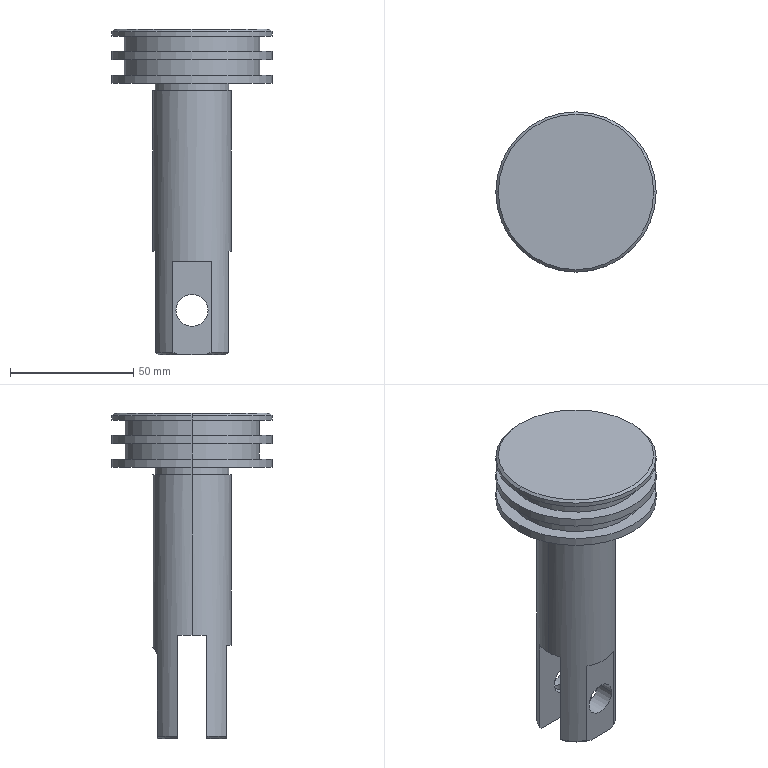Part | SolidWorks | features ICE 9, Chamfer 2, 3DProfileFeature 1, Extrusion 1, Fillet 1, HoleWzd 1 | 1 solid | 42 faces | box 65 x 65 x 132 mm | volume 129865 mm3 | cylinder 21 | plane 15 | cone 6 | commonest cylinder face diameters 65 x6 13 x4 55 x4 3.3 x2 30 x2 32 x2
STEP:
#1=CARTESIAN_POINT('',(1.65,10.,-98.287));
#2=VERTEX_POINT('',#1);
#3=CARTESIAN_POINT('',(-1.65,10.,-98.287));
#4=VERTEX_POINT('',#3);
#5=CARTESIAN_POINT('',(1.65,10.,-98.287));
#6=CARTESIAN_POINT('',(1.65,9.784,-98.287));
#7=CARTESIAN_POINT('',(1.606,9.566,-98.299));
#8=CARTESIAN_POINT('',(1.483,9.268,-98.329));
#9=CARTESIAN_POINT('',(1.431,9.172,-98.341));
#10=CARTESIAN_POINT('',(1.311,8.993,-98.367));
#11=CARTESIAN_POINT('',(1.243,8.91,-98.38));
#12=CARTESIAN_POINT('',(1.091,8.758,-98.408));
#13=CARTESIAN_POINT('',(1.007,8.688,-98.422));
#14=CARTESIAN_POINT('',(0.8287,8.569,-98.448));
#15=CARTESIAN_POINT('',(0.7341,8.518,-98.459));
#16=CARTESIAN_POINT('',(0.4329,8.393,-98.489));
#17=CARTESIAN_POINT('',(0.2181,8.35,-98.5));
#18=CARTESIAN_POINT('',(-0.1083,8.35,-98.5));
#19=CARTESIAN_POINT('',(-0.2157,8.361,-98.497));
#20=CARTESIAN_POINT('',(-0.4277,8.403,-98.487));
#21=CARTESIAN_POINT('',(-0.533,8.435,-98.479));
#22=CARTESIAN_POINT('',(-0.8316,8.559,-98.45));
#23=CARTESIAN_POINT('',(-1.015,8.681,-98.422));
#24=CARTESIAN_POINT('',(-1.318,8.984,-98.367));
#25=CARTESIAN_POINT('',(-1.44,9.167,-98.339));
#26=CARTESIAN_POINT('',(-1.565,9.465,-98.309));
#27=CARTESIAN_POINT('',(-1.597,9.57,-98.301));
#28=CARTESIAN_POINT('',(-1.639,9.783,-98.29));
#29=CARTESIAN_POINT('',(-1.65,9.891,-98.287));
#30=CARTESIAN_POINT('',(-1.65,10.,-98.287));
#31=B_SPLINE_CURVE_WITH_KNOTS('',3,(#5,#6,#7,#8,#9,#10,#11,#12,#13,#14,#15,#16,#17,#18,#19,#20,#21,#22,#23,#24,#25,#26,#27,#28,#29,#30),.UNSPECIFIED.,.F.,.F.,(4,2,2,2,2,2,2,2,2,2,2,2,4),(0.00518,0.005827,0.006151,0.006474,0.006798,0.007122,0.007769,0.008093,0.008416,0.009064,0.009711,0.01003,0.01036),.UNSPECIFIED.);
#32=EDGE_CURVE('',#2,#4,#31,.T.);
#33=ORIENTED_EDGE('',*,*,#32,.F.);
#34=CARTESIAN_POINT('',(1.65,10.,-110.));
#35=VERTEX_POINT('',#34);
#36=CARTESIAN_POINT('',(1.65,10.,-110.));
#37=DIRECTION('',(0.,0.,-1.));
#38=VECTOR('',#37,1000.);
#39=LINE('',#36,#38);
#40=EDGE_CURVE('',#2,#35,#39,.T.);
#41=ORIENTED_EDGE('',*,*,#40,.T.);
#42=CARTESIAN_POINT('',(-1.65,10.,-110.));
#43=VERTEX_POINT('',#42);
#44=CARTESIAN_POINT('',(0.,10.,-110.));
#45=DIRECTION('',(0.,0.,-1.));
#46=DIRECTION('',(-1.,0.,0.));
#47=AXIS2_PLACEMENT_3D('',#44,#45,#46);
#48=CIRCLE('',#47,1.65);
#49=EDGE_CURVE('',#35,#43,#48,.T.);
#50=ORIENTED_EDGE('',*,*,#49,.T.);
#51=CARTESIAN_POINT('',(-1.65,10.,-110.));
#52=DIRECTION('',(0.,0.,-1.));
#53=VECTOR('',#52,1000.);
#54=LINE('',#51,#53);
#55=EDGE_CURVE('',#4,#43,#54,.T.);
#56=ORIENTED_EDGE('',*,*,#55,.F.);
#57=EDGE_LOOP('',(#33,#41,#50,#56));
#58=FACE_OUTER_BOUND('',#57,.T.);
#59=CARTESIAN_POINT('',(0.,10.,-110.));
#60=DIRECTION('',(0.,0.,-1.));
#61=DIRECTION('',(-1.,0.,0.));
#62=AXIS2_PLACEMENT_3D('',#59,#60,#61);
#63=CYLINDRICAL_SURFACE('',#62,1.65);
#64=ADVANCED_FACE('',(#58),#63,.F.);
#65=CARTESIAN_POINT('',(6.5,-14.,-92.));
#66=VERTEX_POINT('',#65);
#67=CARTESIAN_POINT('',(-6.5,-14.,-92.));
#68=VERTEX_POINT('',#67);
#69=CARTESIAN_POINT('',(0.,-14.,-92.));
#70=DIRECTION('',(0.,1.,0.));
#71=DIRECTION('',(-1.,0.,0.));
#72=AXIS2_PLACEMENT_3D('',#69,#70,#71);
#73=CIRCLE('',#72,6.5);
#74=EDGE_CURVE('',#66,#68,#73,.T.);
#75=ORIENTED_EDGE('',*,*,#74,.F.);
#76=CARTESIAN_POINT('',(6.5,-6.,-92.));
#77=VERTEX_POINT('',#76);
#78=CARTESIAN_POINT('',(6.5,-32.5,-92.));
#79=DIRECTION('',(0.,1.,0.));
#80=VECTOR('',#79,1000.);
#81=LINE('',#78,#80);
#82=EDGE_CURVE('',#66,#77,#81,.T.);
#83=ORIENTED_EDGE('',*,*,#82,.T.);
#84=CARTESIAN_POINT('',(-6.5,-6.,-92.));
#85=VERTEX_POINT('',#84);
#86=CARTESIAN_POINT('',(0.,-6.,-92.));
#87=DIRECTION('',(0.,-1.,0.));
#88=DIRECTION('',(1.,0.,0.));
#89=AXIS2_PLACEMENT_3D('',#86,#87,#88);
#90=CIRCLE('',#89,6.5);
#91=EDGE_CURVE('',#85,#77,#90,.T.);
#92=ORIENTED_EDGE('',*,*,#91,.F.);
#93=CARTESIAN_POINT('',(-6.5,-32.5,-92.));
#94=DIRECTION('',(0.,1.,0.));
#95=VECTOR('',#94,1000.);
#96=LINE('',#93,#95);
#97=EDGE_CURVE('',#68,#85,#96,.T.);
#98=ORIENTED_EDGE('',*,*,#97,.F.);
#99=EDGE_LOOP('',(#75,#83,#92,#98));
#100=FACE_OUTER_BOUND('',#99,.T.);
#101=CARTESIAN_POINT('',(0.,-32.5,-92.));
#102=DIRECTION('',(0.,1.,0.));
#103=DIRECTION('',(-1.,0.,0.));
#104=AXIS2_PLACEMENT_3D('',#101,#102,#103);
#105=CYLINDRICAL_SURFACE('',#104,6.5);
#106=ADVANCED_FACE('',(#100),#105,.F.);
#107=CARTESIAN_POINT('',(-1.65,10.,-98.287));
#108=CARTESIAN_POINT('',(-1.65,10.11,-98.287));
#109=CARTESIAN_POINT('',(-1.639,10.217,-98.29));
#110=CARTESIAN_POINT('',(-1.597,10.429,-98.301));
#111=CARTESIAN_POINT('',(-1.565,10.534,-98.309));
#112=CARTESIAN_POINT('',(-1.482,10.733,-98.329));
#113=CARTESIAN_POINT('',(-1.431,10.828,-98.341));
#114=CARTESIAN_POINT('',(-1.312,11.007,-98.367));
#115=CARTESIAN_POINT('',(-1.242,11.091,-98.381));
#116=CARTESIAN_POINT('',(-1.015,11.318,-98.422));
#117=CARTESIAN_POINT('',(-0.8315,11.441,-98.45));
#118=CARTESIAN_POINT('',(-0.4347,11.606,-98.489));
#119=CARTESIAN_POINT('',(-0.2169,11.65,-98.5));
#120=CARTESIAN_POINT('',(0.1074,11.65,-98.5));
#121=CARTESIAN_POINT('',(0.2173,11.639,-98.497));
#122=CARTESIAN_POINT('',(0.4293,11.597,-98.487));
#123=CARTESIAN_POINT('',(0.5324,11.566,-98.479));
#124=CARTESIAN_POINT('',(0.8329,11.441,-98.45));
#125=CARTESIAN_POINT('',(1.014,11.319,-98.422));
#126=CARTESIAN_POINT('',(1.243,11.09,-98.38));
#127=CARTESIAN_POINT('',(1.311,11.007,-98.367));
#128=CARTESIAN_POINT('',(1.431,10.829,-98.341));
#129=CARTESIAN_POINT('',(1.483,10.732,-98.329));
#130=CARTESIAN_POINT('',(1.565,10.533,-98.309));
#131=CARTESIAN_POINT('',(1.597,10.43,-98.301));
#132=CARTESIAN_POINT('',(1.639,10.218,-98.29));
#133=CARTESIAN_POINT('',(1.65,10.108,-98.287));
#134=CARTESIAN_POINT('',(1.65,10.,-98.287));
#135=B_SPLINE_CURVE_WITH_KNOTS('',3,(#107,#108,#109,#110,#111,#112,#113,#114,#115,#116,#117,#118,#119,#120,#121,#122,#123,#124,#125,#126,#127,#128,#129,#130,#131,#132,#133,#134),.UNSPECIFIED.,.F.,.F.,(4,2,2,2,2,2,2,2,2,2,2,2,2,4),(0.,0.0003237,0.0006475,0.0009712,0.001295,0.001942,0.00259,0.002914,0.003237,0.003885,0.004209,0.004532,0.004856,0.00518),.UNSPECIFIED.);
#136=EDGE_CURVE('',#4,#2,#135,.T.);
#137=ORIENTED_EDGE('',*,*,#136,.T.);
#138=ORIENTED_EDGE('',*,*,#32,.T.);
#139=EDGE_LOOP('',(#137,#138));
#140=FACE_BOUND('',#139,.T.);
#141=CARTESIAN_POINT('',(6.5,6.,-92.));
#142=VERTEX_POINT('',#141);
#143=CARTESIAN_POINT('',(-6.5,6.,-92.));
#144=VERTEX_POINT('',#143);
#145=CARTESIAN_POINT('',(0.,6.,-92.));
#146=DIRECTION('',(0.,1.,0.));
#147=DIRECTION('',(-1.,0.,0.));
#148=AXIS2_PLACEMENT_3D('',#145,#146,#147);
#149=CIRCLE('',#148,6.5);
#150=EDGE_CURVE('',#142,#144,#149,.T.);
#151=ORIENTED_EDGE('',*,*,#150,.F.);
#152=CARTESIAN_POINT('',(6.5,14.,-92.));
#153=VERTEX_POINT('',#152);
#154=CARTESIAN_POINT('',(6.5,-32.5,-92.));
#155=DIRECTION('',(0.,1.,0.));
#156=VECTOR('',#155,1000.);
#157=LINE('',#154,#156);
#158=EDGE_CURVE('',#142,#153,#157,.T.);
#159=ORIENTED_EDGE('',*,*,#158,.T.);
#160=CARTESIAN_POINT('',(-6.5,14.,-92.));
#161=VERTEX_POINT('',#160);
#162=CARTESIAN_POINT('',(0.,14.,-92.));
#163=DIRECTION('',(0.,1.,0.));
#164=DIRECTION('',(-1.,0.,0.));
#165=AXIS2_PLACEMENT_3D('',#162,#163,#164);
#166=CIRCLE('',#165,6.5);
#167=EDGE_CURVE('',#153,#161,#166,.T.);
#168=ORIENTED_EDGE('',*,*,#167,.T.);
#169=CARTESIAN_POINT('',(-6.5,-32.5,-92.));
#170=DIRECTION('',(0.,1.,0.));
#171=VECTOR('',#170,1000.);
#172=LINE('',#169,#171);
#173=EDGE_CURVE('',#144,#161,#172,.T.);
#174=ORIENTED_EDGE('',*,*,#173,.F.);
#175=EDGE_LOOP('',(#151,#159,#168,#174));
#176=FACE_OUTER_BOUND('',#175,.T.);
#177=CARTESIAN_POINT('',(0.,-32.5,-92.));
#178=DIRECTION('',(0.,1.,0.));
#179=DIRECTION('',(-1.,0.,0.));
#180=AXIS2_PLACEMENT_3D('',#177,#178,#179);
#181=CYLINDRICAL_SURFACE('',#180,6.5);
#182=ADVANCED_FACE('',(#140,#176),#181,.F.);
#183=CARTESIAN_POINT('',(-16.,0.,-68.));
#184=VERTEX_POINT('',#183);
#185=CARTESIAN_POINT('',(-14.832,6.,-68.));
#186=VERTEX_POINT('',#185);
#187=CARTESIAN_POINT('',(0.,0.,-68.));
#188=DIRECTION('',(0.,0.,-1.));
#189=DIRECTION('',(-1.,0.,0.));
#190=AXIS2_PLACEMENT_3D('',#187,#188,#189);
#191=CIRCLE('',#190,16.);
#192=EDGE_CURVE('',#184,#186,#191,.T.);
#193=ORIENTED_EDGE('',*,*,#192,.F.);
#194=CARTESIAN_POINT('',(-16.,0.,-3.));
#195=VERTEX_POINT('',#194);
#196=CARTESIAN_POINT('',(-16.,0.,-110.));
#197=DIRECTION('',(0.,0.,1.));
#198=VECTOR('',#197,1000.);
#199=LINE('',#196,#198);
#200=EDGE_CURVE('',#184,#195,#199,.T.);
#201=ORIENTED_EDGE('',*,*,#200,.T.);
#202=CARTESIAN_POINT('',(16.,0.,-3.));
#203=VERTEX_POINT('',#202);
#204=CARTESIAN_POINT('',(0.,0.,-3.));
#205=DIRECTION('',(0.,0.,-1.));
#206=DIRECTION('',(-1.,0.,0.));
#207=AXIS2_PLACEMENT_3D('',#204,#205,#206);
#208=CIRCLE('',#207,16.);
#209=EDGE_CURVE('',#195,#203,#208,.T.);
#210=ORIENTED_EDGE('',*,*,#209,.T.);
#211=CARTESIAN_POINT('',(16.,0.,-68.));
#212=VERTEX_POINT('',#211);
#213=CARTESIAN_POINT('',(16.,0.,-110.));
#214=DIRECTION('',(0.,0.,1.));
#215=VECTOR('',#214,1000.);
#216=LINE('',#213,#215);
#217=EDGE_CURVE('',#212,#203,#216,.T.);
#218=ORIENTED_EDGE('',*,*,#217,.F.);
#219=CARTESIAN_POINT('',(14.832,6.,-68.));
#220=VERTEX_POINT('',#219);
#221=CARTESIAN_POINT('',(0.,0.,-68.));
#222=DIRECTION('',(0.,0.,-1.));
#223=DIRECTION('',(-1.,0.,0.));
#224=AXIS2_PLACEMENT_3D('',#221,#222,#223);
#225=CIRCLE('',#224,16.);
#226=EDGE_CURVE('',#220,#212,#225,.T.);
#227=ORIENTED_EDGE('',*,*,#226,.F.);
#228=CARTESIAN_POINT('',(14.832,6.,-109.));
#229=VERTEX_POINT('',#228);
#230=CARTESIAN_POINT('',(14.832,6.,-110.));
#231=DIRECTION('',(0.,0.,-1.));
#232=VECTOR('',#231,1000.);
#233=LINE('',#230,#232);
#234=EDGE_CURVE('',#220,#229,#233,.T.);
#235=ORIENTED_EDGE('',*,*,#234,.T.);
#236=CARTESIAN_POINT('',(7.746,14.,-109.));
#237=VERTEX_POINT('',#236);
#238=CARTESIAN_POINT('',(0.,0.,-109.));
#239=DIRECTION('',(0.,0.,1.));
#240=DIRECTION('',(-1.,0.,0.));
#241=AXIS2_PLACEMENT_3D('',#238,#239,#240);
#242=CIRCLE('',#241,16.);
#243=EDGE_CURVE('',#229,#237,#242,.T.);
#244=ORIENTED_EDGE('',*,*,#243,.T.);
#245=CARTESIAN_POINT('',(7.746,14.,-77.));
#246=VERTEX_POINT('',#245);
#247=CARTESIAN_POINT('',(7.746,14.,-110.));
#248=DIRECTION('',(0.,0.,1.));
#249=VECTOR('',#248,1000.);
#250=LINE('',#247,#249);
#251=EDGE_CURVE('',#237,#246,#250,.T.);
#252=ORIENTED_EDGE('',*,*,#251,.T.);
#253=CARTESIAN_POINT('',(-7.746,14.,-77.));
#254=VERTEX_POINT('',#253);
#255=CARTESIAN_POINT('',(7.746,14.,-77.));
#256=CARTESIAN_POINT('',(7.746,14.,-76.791));
#257=CARTESIAN_POINT('',(7.722,14.013,-76.586));
#258=CARTESIAN_POINT('',(7.632,14.063,-76.186));
#259=CARTESIAN_POINT('',(7.564,14.099,-75.99));
#260=CARTESIAN_POINT('',(7.394,14.189,-75.624));
#261=CARTESIAN_POINT('',(7.291,14.243,-75.451));
#262=CARTESIAN_POINT('',(7.057,14.36,-75.129));
#263=CARTESIAN_POINT('',(6.928,14.423,-74.982));
#264=CARTESIAN_POINT('',(6.65,14.554,-74.708));
#265=CARTESIAN_POINT('',(6.499,14.622,-74.582));
#266=CARTESIAN_POINT('',(6.184,14.758,-74.35));
#267=CARTESIAN_POINT('',(6.02,14.825,-74.246));
#268=CARTESIAN_POINT('',(5.514,15.024,-73.959));
#269=CARTESIAN_POINT('',(5.155,15.152,-73.803));
#270=CARTESIAN_POINT('',(4.406,15.386,-73.54));
#271=CARTESIAN_POINT('',(4.024,15.491,-73.436));
#272=CARTESIAN_POINT('',(3.245,15.672,-73.266));
#273=CARTESIAN_POINT('',(2.85,15.749,-73.2));
#274=CARTESIAN_POINT('',(2.047,15.874,-73.097));
#275=CARTESIAN_POINT('',(1.638,15.921,-73.06));
#276=CARTESIAN_POINT('',(0.8181,15.984,-73.012));
#277=CARTESIAN_POINT('',(0.4067,16.,-73.));
#278=CARTESIAN_POINT('',(-0.8311,16.,-73.));
#279=CARTESIAN_POINT('',(-1.643,15.936,-73.046));
#280=CARTESIAN_POINT('',(-2.839,15.751,-73.198));
#281=CARTESIAN_POINT('',(-3.235,15.675,-73.264));
#282=CARTESIAN_POINT('',(-4.017,15.493,-73.434));
#283=CARTESIAN_POINT('',(-4.405,15.387,-73.54));
#284=CARTESIAN_POINT('',(-5.15,15.154,-73.801));
#285=CARTESIAN_POINT('',(-5.511,15.026,-73.957));
#286=CARTESIAN_POINT('',(-6.192,14.758,-74.343));
#287=CARTESIAN_POINT('',(-6.507,14.62,-74.569));
#288=CARTESIAN_POINT('',(-6.927,14.424,-74.98));
#289=CARTESIAN_POINT('',(-7.058,14.36,-75.13));
#290=CARTESIAN_POINT('',(-7.29,14.243,-75.45));
#291=CARTESIAN_POINT('',(-7.392,14.19,-75.621));
#292=CARTESIAN_POINT('',(-7.564,14.099,-75.99));
#293=CARTESIAN_POINT('',(-7.631,14.063,-76.182));
#294=CARTESIAN_POINT('',(-7.722,14.013,-76.582));
#295=CARTESIAN_POINT('',(-7.746,14.,-76.791));
#296=CARTESIAN_POINT('',(-7.746,14.,-77.));
#297=B_SPLINE_CURVE_WITH_KNOTS('',3,(#255,#256,#257,#258,#259,#260,#261,#262,#263,#264,#265,#266,#267,#268,#269,#270,#271,#272,#273,#274,#275,#276,#277,#278,#279,#280,#281,#282,#283,#284,#285,#286,#287,#288,#289,#290,#291,#292,#293,#294,#295,#296),.UNSPECIFIED.,.F.,.F.,(4,2,2,2,2,2,2,2,2,2,2,2,2,2,2,2,2,2,2,2,4),(-0.009753,-0.009143,-0.008533,-0.007923,-0.007313,-0.006703,-0.006093,-0.004873,-0.003654,-0.002434,-0.001214,0.000005848,0.002446,0.003665,0.004885,0.006105,0.007325,0.007935,0.008545,0.009155,0.009765),.UNSPECIFIED.);
#298=EDGE_CURVE('',#246,#254,#297,.T.);
#299=ORIENTED_EDGE('',*,*,#298,.T.);
#300=CARTESIAN_POINT('',(-7.746,14.,-109.));
#301=VERTEX_POINT('',#300);
#302=CARTESIAN_POINT('',(-7.746,14.,-110.));
#303=DIRECTION('',(0.,0.,-1.));
#304=VECTOR('',#303,1000.);
#305=LINE('',#302,#304);
#306=EDGE_CURVE('',#254,#301,#305,.T.);
#307=ORIENTED_EDGE('',*,*,#306,.T.);
#308=CARTESIAN_POINT('',(-14.832,6.,-109.));
#309=VERTEX_POINT('',#308);
#310=CARTESIAN_POINT('',(0.,0.,-109.));
#311=DIRECTION('',(0.,0.,1.));
#312=DIRECTION('',(-1.,0.,0.));
#313=AXIS2_PLACEMENT_3D('',#310,#311,#312);
#314=CIRCLE('',#313,16.);
#315=EDGE_CURVE('',#301,#309,#314,.T.);
#316=ORIENTED_EDGE('',*,*,#315,.T.);
#317=CARTESIAN_POINT('',(-14.832,6.,-110.));
#318=DIRECTION('',(0.,0.,1.));
#319=VECTOR('',#318,1000.);
#320=LINE('',#317,#319);
#321=EDGE_CURVE('',#309,#186,#320,.T.);
#322=ORIENTED_EDGE('',*,*,#321,.T.);
#323=EDGE_LOOP('',(#193,#201,#210,#218,#227,#235,#244,#252,#299,#307,#316,#322));
#324=FACE_OUTER_BOUND('',#323,.T.);
#325=CARTESIAN_POINT('',(0.,0.,-110.));
#326=DIRECTION('',(0.,0.,1.));
#327=DIRECTION('',(1.,0.,0.));
#328=AXIS2_PLACEMENT_3D('',#325,#326,#327);
#329=CYLINDRICAL_SURFACE('',#328,16.);
#330=ADVANCED_FACE('',(#324),#329,.T.);
#331=CARTESIAN_POINT('',(-15.,0.,-3.));
#332=VERTEX_POINT('',#331);
#333=CARTESIAN_POINT('',(15.,0.,-3.));
#334=VERTEX_POINT('',#333);
#335=CARTESIAN_POINT('',(0.,0.,-3.));
#336=DIRECTION('',(0.,0.,-1.));
#337=DIRECTION('',(-1.,0.,0.));
#338=AXIS2_PLACEMENT_3D('',#335,#336,#337);
#339=CIRCLE('',#338,15.);
#340=EDGE_CURVE('',#332,#334,#339,.T.);
#341=ORIENTED_EDGE('',*,*,#340,.F.);
#342=CARTESIAN_POINT('',(-15.,0.,0.));
#343=VERTEX_POINT('',#342);
#344=CARTESIAN_POINT('',(-15.,0.,-3.));
#345=DIRECTION('',(0.,0.,1.));
#346=VECTOR('',#345,1000.);
#347=LINE('',#344,#346);
#348=EDGE_CURVE('',#332,#343,#347,.T.);
#349=ORIENTED_EDGE('',*,*,#348,.T.);
#350=CARTESIAN_POINT('',(15.,0.,0.));
#351=VERTEX_POINT('',#350);
#352=CARTESIAN_POINT('',(0.,0.,0.));
#353=DIRECTION('',(0.,0.,-1.));
#354=DIRECTION('',(-1.,0.,0.));
#355=AXIS2_PLACEMENT_3D('',#352,#353,#354);
#356=CIRCLE('',#355,15.);
#357=EDGE_CURVE('',#343,#351,#356,.T.);
#358=ORIENTED_EDGE('',*,*,#357,.T.);
#359=CARTESIAN_POINT('',(15.,0.,-3.));
#360=DIRECTION('',(0.,0.,1.));
#361=VECTOR('',#360,1000.);
#362=LINE('',#359,#361);
#363=EDGE_CURVE('',#334,#351,#362,.T.);
#364=ORIENTED_EDGE('',*,*,#363,.F.);
#365=EDGE_LOOP('',(#341,#349,#358,#364));
#366=FACE_OUTER_BOUND('',#365,.T.);
#367=CARTESIAN_POINT('',(0.,0.,-3.));
#368=DIRECTION('',(0.,0.,1.));
#369=DIRECTION('',(1.,0.,0.));
#370=AXIS2_PLACEMENT_3D('',#367,#368,#369);
#371=CYLINDRICAL_SURFACE('',#370,15.);
#372=ADVANCED_FACE('',(#366),#371,.T.);
#373=CARTESIAN_POINT('',(31.5,0.,22.));
#374=VERTEX_POINT('',#373);
#375=CARTESIAN_POINT('',(-31.5,0.,22.));
#376=VERTEX_POINT('',#375);
#377=CARTESIAN_POINT('',(0.,0.,22.));
#378=DIRECTION('',(0.,0.,1.));
#379=DIRECTION('',(1.,0.,0.));
#380=AXIS2_PLACEMENT_3D('',#377,#378,#379);
#381=CIRCLE('',#380,31.5);
#382=EDGE_CURVE('',#374,#376,#381,.T.);
#383=ORIENTED_EDGE('',*,*,#382,.F.);
#384=CARTESIAN_POINT('',(32.5,0.,21.));
#385=VERTEX_POINT('',#384);
#386=CARTESIAN_POINT('',(31.5,0.,22.));
#387=DIRECTION('',(0.7071,0.,-0.7071));
#388=VECTOR('',#387,1000.);
#389=LINE('',#386,#388);
#390=EDGE_CURVE('',#374,#385,#389,.T.);
#391=ORIENTED_EDGE('',*,*,#390,.T.);
#392=CARTESIAN_POINT('',(-32.5,0.,21.));
#393=VERTEX_POINT('',#392);
#394=CARTESIAN_POINT('',(0.,0.,21.));
#395=DIRECTION('',(0.,0.,-1.));
#396=DIRECTION('',(1.,0.,0.));
#397=AXIS2_PLACEMENT_3D('',#394,#395,#396);
#398=CIRCLE('',#397,32.5);
#399=EDGE_CURVE('',#393,#385,#398,.T.);
#400=ORIENTED_EDGE('',*,*,#399,.F.);
#401=CARTESIAN_POINT('',(-31.5,0.,22.));
#402=DIRECTION('',(-0.7071,0.,-0.7071));
#403=VECTOR('',#402,1000.);
#404=LINE('',#401,#403);
#405=EDGE_CURVE('',#376,#393,#404,.T.);
#406=ORIENTED_EDGE('',*,*,#405,.F.);
#407=EDGE_LOOP('',(#383,#391,#400,#406));
#408=FACE_OUTER_BOUND('',#407,.T.);
#409=CARTESIAN_POINT('',(0.,0.,22.));
#410=DIRECTION('',(0.,0.,-1.));
#411=DIRECTION('',(-1.,0.,0.));
#412=AXIS2_PLACEMENT_3D('',#409,#410,#411);
#413=CONICAL_SURFACE('',#412,31.5,0.7854);
#414=ADVANCED_FACE('',(#408),#413,.T.);
#415=ORIENTED_EDGE('',*,*,#399,.T.);
#416=CARTESIAN_POINT('',(32.5,0.,19.2));
#417=VERTEX_POINT('',#416);
#418=CARTESIAN_POINT('',(32.5,0.,22.));
#419=DIRECTION('',(0.,0.,-1.));
#420=VECTOR('',#419,1000.);
#421=LINE('',#418,#420);
#422=EDGE_CURVE('',#385,#417,#421,.T.);
#423=ORIENTED_EDGE('',*,*,#422,.T.);
#424=CARTESIAN_POINT('',(-32.5,0.,19.2));
#425=VERTEX_POINT('',#424);
#426=CARTESIAN_POINT('',(0.,0.,19.2));
#427=DIRECTION('',(0.,0.,1.));
#428=DIRECTION('',(1.,0.,0.));
#429=AXIS2_PLACEMENT_3D('',#426,#427,#428);
#430=CIRCLE('',#429,32.5);
#431=EDGE_CURVE('',#417,#425,#430,.T.);
#432=ORIENTED_EDGE('',*,*,#431,.T.);
#433=CARTESIAN_POINT('',(-32.5,0.,22.));
#434=DIRECTION('',(0.,0.,-1.));
#435=VECTOR('',#434,1000.);
#436=LINE('',#433,#435);
#437=EDGE_CURVE('',#393,#425,#436,.T.);
#438=ORIENTED_EDGE('',*,*,#437,.F.);
#439=EDGE_LOOP('',(#415,#423,#432,#438));
#440=FACE_OUTER_BOUND('',#439,.T.);
#441=CARTESIAN_POINT('',(0.,0.,22.));
#442=DIRECTION('',(0.,0.,-1.));
#443=DIRECTION('',(-1.,0.,0.));
#444=AXIS2_PLACEMENT_3D('',#441,#442,#443);
#445=CYLINDRICAL_SURFACE('',#444,32.5);
#446=ADVANCED_FACE('',(#440),#445,.T.);
#447=CARTESIAN_POINT('',(27.5,0.,19.2));
#448=VERTEX_POINT('',#447);
#449=CARTESIAN_POINT('',(-27.5,0.,19.2));
#450=VERTEX_POINT('',#449);
#451=CARTESIAN_POINT('',(0.,0.,19.2));
#452=DIRECTION('',(0.,0.,1.));
#453=DIRECTION('',(1.,0.,0.));
#454=AXIS2_PLACEMENT_3D('',#451,#452,#453);
#455=CIRCLE('',#454,27.5);
#456=EDGE_CURVE('',#448,#450,#455,.T.);
#457=ORIENTED_EDGE('',*,*,#456,.F.);
#458=CARTESIAN_POINT('',(27.5,0.,13.));
#459=VERTEX_POINT('',#458);
#460=CARTESIAN_POINT('',(27.5,0.,19.2));
#461=DIRECTION('',(0.,0.,-1.));
#462=VECTOR('',#461,1000.);
#463=LINE('',#460,#462);
#464=EDGE_CURVE('',#448,#459,#463,.T.);
#465=ORIENTED_EDGE('',*,*,#464,.T.);
#466=CARTESIAN_POINT('',(-27.5,0.,13.));
#467=VERTEX_POINT('',#466);
#468=CARTESIAN_POINT('',(0.,0.,13.));
#469=DIRECTION('',(0.,0.,1.));
#470=DIRECTION('',(1.,0.,0.));
#471=AXIS2_PLACEMENT_3D('',#468,#469,#470);
#472=CIRCLE('',#471,27.5);
#473=EDGE_CURVE('',#459,#467,#472,.T.);
#474=ORIENTED_EDGE('',*,*,#473,.T.);
#475=CARTESIAN_POINT('',(-27.5,0.,19.2));
#476=DIRECTION('',(0.,0.,-1.));
#477=VECTOR('',#476,1000.);
#478=LINE('',#475,#477);
#479=EDGE_CURVE('',#450,#467,#478,.T.);
#480=ORIENTED_EDGE('',*,*,#479,.F.);
#481=EDGE_LOOP('',(#457,#465,#474,#480));
#482=FACE_OUTER_BOUND('',#481,.T.);
#483=CARTESIAN_POINT('',(0.,0.,19.2));
#484=DIRECTION('',(0.,0.,-1.));
#485=DIRECTION('',(-1.,0.,0.));
#486=AXIS2_PLACEMENT_3D('',#483,#484,#485);
#487=CYLINDRICAL_SURFACE('',#486,27.5);
#488=ADVANCED_FACE('',(#482),#487,.T.);
#489=CARTESIAN_POINT('',(32.5,0.,13.));
#490=VERTEX_POINT('',#489);
#491=CARTESIAN_POINT('',(-32.5,0.,13.));
#492=VERTEX_POINT('',#491);
#493=CARTESIAN_POINT('',(0.,0.,13.));
#494=DIRECTION('',(0.,0.,1.));
#495=DIRECTION('',(1.,0.,0.));
#496=AXIS2_PLACEMENT_3D('',#493,#494,#495);
#497=CIRCLE('',#496,32.5);
#498=EDGE_CURVE('',#490,#492,#497,.T.);
#499=ORIENTED_EDGE('',*,*,#498,.F.);
#500=CARTESIAN_POINT('',(32.5,0.,9.6));
#501=VERTEX_POINT('',#500);
#502=CARTESIAN_POINT('',(32.5,0.,13.));
#503=DIRECTION('',(0.,0.,-1.));
#504=VECTOR('',#503,1000.);
#505=LINE('',#502,#504);
#506=EDGE_CURVE('',#490,#501,#505,.T.);
#507=ORIENTED_EDGE('',*,*,#506,.T.);
#508=CARTESIAN_POINT('',(-32.5,0.,9.6));
#509=VERTEX_POINT('',#508);
#510=CARTESIAN_POINT('',(0.,0.,9.6));
#511=DIRECTION('',(0.,0.,1.));
#512=DIRECTION('',(1.,0.,0.));
#513=AXIS2_PLACEMENT_3D('',#510,#511,#512);
#514=CIRCLE('',#513,32.5);
#515=EDGE_CURVE('',#501,#509,#514,.T.);
#516=ORIENTED_EDGE('',*,*,#515,.T.);
#517=CARTESIAN_POINT('',(-32.5,0.,13.));
#518=DIRECTION('',(0.,0.,-1.));
#519=VECTOR('',#518,1000.);
#520=LINE('',#517,#519);
#521=EDGE_CURVE('',#492,#509,#520,.T.);
#522=ORIENTED_EDGE('',*,*,#521,.F.);
#523=EDGE_LOOP('',(#499,#507,#516,#522));
#524=FACE_OUTER_BOUND('',#523,.T.);
#525=CARTESIAN_POINT('',(0.,0.,13.));
#526=DIRECTION('',(0.,0.,-1.));
#527=DIRECTION('',(-1.,0.,0.));
#528=AXIS2_PLACEMENT_3D('',#525,#526,#527);
#529=CYLINDRICAL_SURFACE('',#528,32.5);
#530=ADVANCED_FACE('',(#524),#529,.T.);
#531=CARTESIAN_POINT('',(27.5,0.,9.6));
#532=VERTEX_POINT('',#531);
#533=CARTESIAN_POINT('',(-27.5,0.,9.6));
#534=VERTEX_POINT('',#533);
#535=CARTESIAN_POINT('',(0.,0.,9.6));
#536=DIRECTION('',(0.,0.,1.));
#537=DIRECTION('',(1.,0.,0.));
#538=AXIS2_PLACEMENT_3D('',#535,#536,#537);
#539=CIRCLE('',#538,27.5);
#540=EDGE_CURVE('',#532,#534,#539,.T.);
#541=ORIENTED_EDGE('',*,*,#540,.F.);
#542=CARTESIAN_POINT('',(27.5,0.,3.4));
#543=VERTEX_POINT('',#542);
#544=CARTESIAN_POINT('',(27.5,0.,9.6));
#545=DIRECTION('',(0.,0.,-1.));
#546=VECTOR('',#545,1000.);
#547=LINE('',#544,#546);
#548=EDGE_CURVE('',#532,#543,#547,.T.);
#549=ORIENTED_EDGE('',*,*,#548,.T.);
#550=CARTESIAN_POINT('',(-27.5,0.,3.4));
#551=VERTEX_POINT('',#550);
#552=CARTESIAN_POINT('',(0.,0.,3.4));
#553=DIRECTION('',(0.,0.,1.));
#554=DIRECTION('',(1.,0.,0.));
#555=AXIS2_PLACEMENT_3D('',#552,#553,#554);
#556=CIRCLE('',#555,27.5);
#557=EDGE_CURVE('',#543,#551,#556,.T.);
#558=ORIENTED_EDGE('',*,*,#557,.T.);
#559=CARTESIAN_POINT('',(-27.5,0.,9.6));
#560=DIRECTION('',(0.,0.,-1.));
#561=VECTOR('',#560,1000.);
#562=LINE('',#559,#561);
#563=EDGE_CURVE('',#534,#551,#562,.T.);
#564=ORIENTED_EDGE('',*,*,#563,.F.);
#565=EDGE_LOOP('',(#541,#549,#558,#564));
#566=FACE_OUTER_BOUND('',#565,.T.);
#567=CARTESIAN_POINT('',(0.,0.,9.6));
#568=DIRECTION('',(0.,0.,-1.));
#569=DIRECTION('',(-1.,0.,0.));
#570=AXIS2_PLACEMENT_3D('',#567,#568,#569);
#571=CYLINDRICAL_SURFACE('',#570,27.5);
#572=ADVANCED_FACE('',(#566),#571,.T.);
#573=CARTESIAN_POINT('',(32.5,0.,3.4));
#574=VERTEX_POINT('',#573);
#575=CARTESIAN_POINT('',(-32.5,0.,3.4));
#576=VERTEX_POINT('',#575);
#577=CARTESIAN_POINT('',(0.,0.,3.4));
#578=DIRECTION('',(0.,0.,1.));
#579=DIRECTION('',(1.,0.,0.));
#580=AXIS2_PLACEMENT_3D('',#577,#578,#579);
#581=CIRCLE('',#580,32.5);
#582=EDGE_CURVE('',#574,#576,#581,.T.);
#583=ORIENTED_EDGE('',*,*,#582,.F.);
#584=CARTESIAN_POINT('',(32.5,0.,0.));
#585=VERTEX_POINT('',#584);
#586=CARTESIAN_POINT('',(32.5,0.,3.4));
#587=DIRECTION('',(0.,0.,-1.));
#588=VECTOR('',#587,1000.);
#589=LINE('',#586,#588);
#590=EDGE_CURVE('',#574,#585,#589,.T.);
#591=ORIENTED_EDGE('',*,*,#590,.T.);
#592=CARTESIAN_POINT('',(-32.5,0.,0.));
#593=VERTEX_POINT('',#592);
#594=CARTESIAN_POINT('',(0.,0.,0.));
#595=DIRECTION('',(0.,0.,1.));
#596=DIRECTION('',(1.,0.,0.));
#597=AXIS2_PLACEMENT_3D('',#594,#595,#596);
#598=CIRCLE('',#597,32.5);
#599=EDGE_CURVE('',#585,#593,#598,.T.);
#600=ORIENTED_EDGE('',*,*,#599,.T.);
#601=CARTESIAN_POINT('',(-32.5,0.,3.4));
#602=DIRECTION('',(0.,0.,-1.));
#603=VECTOR('',#602,1000.);
#604=LINE('',#601,#603);
#605=EDGE_CURVE('',#576,#593,#604,.T.);
#606=ORIENTED_EDGE('',*,*,#605,.F.);
#607=EDGE_LOOP('',(#583,#591,#600,#606));
#608=FACE_OUTER_BOUND('',#607,.T.);
#609=CARTESIAN_POINT('',(0.,0.,3.4));
#610=DIRECTION('',(0.,0.,-1.));
#611=DIRECTION('',(-1.,0.,0.));
#612=AXIS2_PLACEMENT_3D('',#609,#610,#611);
#613=CYLINDRICAL_SURFACE('',#612,32.5);
#614=ADVANCED_FACE('',(#608),#613,.T.);
#615=CARTESIAN_POINT('',(0.,10.,-110.));
#616=DIRECTION('',(0.,0.,-1.));
#617=DIRECTION('',(-1.,0.,0.));
#618=AXIS2_PLACEMENT_3D('',#615,#616,#617);
#619=CIRCLE('',#618,1.65);
#620=EDGE_CURVE('',#43,#35,#619,.T.);
#621=ORIENTED_EDGE('',*,*,#620,.F.);
#622=ORIENTED_EDGE('',*,*,#49,.F.);
#623=EDGE_LOOP('',(#621,#622));
#624=FACE_BOUND('',#623,.T.);
#625=CARTESIAN_POINT('',(-13.748,6.,-110.));
#626=VERTEX_POINT('',#625);
#627=CARTESIAN_POINT('',(13.748,6.,-110.));
#628=VERTEX_POINT('',#627);
#629=CARTESIAN_POINT('',(0.,6.,-110.));
#630=DIRECTION('',(1.,0.,0.));
#631=VECTOR('',#630,1000.);
#632=LINE('',#629,#631);
#633=EDGE_CURVE('',#626,#628,#632,.T.);
#634=ORIENTED_EDGE('',*,*,#633,.F.);
#635=CARTESIAN_POINT('',(-5.385,14.,-110.));
#636=VERTEX_POINT('',#635);
#637=CARTESIAN_POINT('',(0.,0.,-110.));
#638=DIRECTION('',(0.,0.,-1.));
#639=DIRECTION('',(-1.,0.,0.));
#640=AXIS2_PLACEMENT_3D('',#637,#638,#639);
#641=CIRCLE('',#640,15.);
#642=EDGE_CURVE('',#626,#636,#641,.T.);
#643=ORIENTED_EDGE('',*,*,#642,.T.);
#644=CARTESIAN_POINT('',(5.385,14.,-110.));
#645=VERTEX_POINT('',#644);
#646=CARTESIAN_POINT('',(-18.152,14.,-110.));
#647=DIRECTION('',(-1.,0.,0.));
#648=VECTOR('',#647,1000.);
#649=LINE('',#646,#648);
#650=EDGE_CURVE('',#645,#636,#649,.T.);
#651=ORIENTED_EDGE('',*,*,#650,.F.);
#652=CARTESIAN_POINT('',(0.,0.,-110.));
#653=DIRECTION('',(0.,0.,-1.));
#654=DIRECTION('',(-1.,0.,0.));
#655=AXIS2_PLACEMENT_3D('',#652,#653,#654);
#656=CIRCLE('',#655,15.);
#657=EDGE_CURVE('',#645,#628,#656,.T.);
#658=ORIENTED_EDGE('',*,*,#657,.T.);
#659=EDGE_LOOP('',(#634,#643,#651,#658));
#660=FACE_OUTER_BOUND('',#659,.T.);
#661=CARTESIAN_POINT('',(0.,0.,-110.));
#662=DIRECTION('',(0.,0.,-1.));
#663=DIRECTION('',(-1.,0.,0.));
#664=AXIS2_PLACEMENT_3D('',#661,#662,#663);
#665=PLANE('',#664);
#666=ADVANCED_FACE('',(#624,#660),#665,.T.);
#667=ORIENTED_EDGE('',*,*,#590,.F.);
#668=CARTESIAN_POINT('',(0.,0.,3.4));
#669=DIRECTION('',(0.,0.,1.));
#670=DIRECTION('',(1.,0.,0.));
#671=AXIS2_PLACEMENT_3D('',#668,#669,#670);
#672=CIRCLE('',#671,32.5);
#673=EDGE_CURVE('',#576,#574,#672,.T.);
#674=ORIENTED_EDGE('',*,*,#673,.F.);
#675=ORIENTED_EDGE('',*,*,#605,.T.);
#676=CARTESIAN_POINT('',(0.,0.,0.));
#677=DIRECTION('',(0.,0.,1.));
#678=DIRECTION('',(1.,0.,0.));
#679=AXIS2_PLACEMENT_3D('',#676,#677,#678);
#680=CIRCLE('',#679,32.5);
#681=EDGE_CURVE('',#593,#585,#680,.T.);
#682=ORIENTED_EDGE('',*,*,#681,.T.);
#683=EDGE_LOOP('',(#667,#674,#675,#682));
#684=FACE_OUTER_BOUND('',#683,.T.);
#685=CARTESIAN_POINT('',(0.,0.,3.4));
#686=DIRECTION('',(0.,0.,-1.));
#687=DIRECTION('',(-1.,0.,0.));
#688=AXIS2_PLACEMENT_3D('',#685,#686,#687);
#689=CYLINDRICAL_SURFACE('',#688,32.5);
#690=ADVANCED_FACE('',(#684),#689,.T.);
#691=CARTESIAN_POINT('',(0.,0.,3.4));
#692=DIRECTION('',(0.,0.,1.));
#693=DIRECTION('',(1.,0.,0.));
#694=AXIS2_PLACEMENT_3D('',#691,#692,#693);
#695=CIRCLE('',#694,27.5);
#696=EDGE_CURVE('',#551,#543,#695,.T.);
#697=ORIENTED_EDGE('',*,*,#696,.F.);
#698=ORIENTED_EDGE('',*,*,#557,.F.);
#699=EDGE_LOOP('',(#697,#698));
#700=FACE_BOUND('',#699,.T.);
#701=ORIENTED_EDGE('',*,*,#673,.T.);
#702=ORIENTED_EDGE('',*,*,#582,.T.);
#703=EDGE_LOOP('',(#701,#702));
#704=FACE_OUTER_BOUND('',#703,.T.);
#705=CARTESIAN_POINT('',(0.,0.,3.4));
#706=DIRECTION('',(0.,0.,1.));
#707=DIRECTION('',(1.,0.,0.));
#708=AXIS2_PLACEMENT_3D('',#705,#706,#707);
#709=PLANE('',#708);
#710=ADVANCED_FACE('',(#700,#704),#709,.T.);
#711=CARTESIAN_POINT('',(0.,0.,0.));
#712=DIRECTION('',(0.,0.,-1.));
#713=DIRECTION('',(-1.,0.,0.));
#714=AXIS2_PLACEMENT_3D('',#711,#712,#713);
#715=CIRCLE('',#714,15.);
#716=EDGE_CURVE('',#351,#343,#715,.T.);
#717=ORIENTED_EDGE('',*,*,#716,.F.);
#718=ORIENTED_EDGE('',*,*,#357,.F.);
#719=EDGE_LOOP('',(#717,#718));
#720=FACE_BOUND('',#719,.T.);
#721=ORIENTED_EDGE('',*,*,#681,.F.);
#722=ORIENTED_EDGE('',*,*,#599,.F.);
#723=EDGE_LOOP('',(#721,#722));
#724=FACE_OUTER_BOUND('',#723,.T.);
#725=CARTESIAN_POINT('',(0.,0.,0.));
#726=DIRECTION('',(0.,0.,1.));
#727=DIRECTION('',(1.,0.,0.));
#728=AXIS2_PLACEMENT_3D('',#725,#726,#727);
#729=PLANE('',#728);
#730=ADVANCED_FACE('',(#720,#724),#729,.F.);
#731=ORIENTED_EDGE('',*,*,#548,.F.);
#732=CARTESIAN_POINT('',(0.,0.,9.6));
#733=DIRECTION('',(0.,0.,1.));
#734=DIRECTION('',(1.,0.,0.));
#735=AXIS2_PLACEMENT_3D('',#732,#733,#734);
#736=CIRCLE('',#735,27.5);
#737=EDGE_CURVE('',#534,#532,#736,.T.);
#738=ORIENTED_EDGE('',*,*,#737,.F.);
#739=ORIENTED_EDGE('',*,*,#563,.T.);
#740=ORIENTED_EDGE('',*,*,#696,.T.);
#741=EDGE_LOOP('',(#731,#738,#739,#740));
#742=FACE_OUTER_BOUND('',#741,.T.);
#743=CARTESIAN_POINT('',(0.,0.,9.6));
#744=DIRECTION('',(0.,0.,-1.));
#745=DIRECTION('',(-1.,0.,0.));
#746=AXIS2_PLACEMENT_3D('',#743,#744,#745);
#747=CYLINDRICAL_SURFACE('',#746,27.5);
#748=ADVANCED_FACE('',(#742),#747,.T.);
#749=ORIENTED_EDGE('',*,*,#506,.F.);
#750=CARTESIAN_POINT('',(0.,0.,13.));
#751=DIRECTION('',(0.,0.,1.));
#752=DIRECTION('',(1.,0.,0.));
#753=AXIS2_PLACEMENT_3D('',#750,#751,#752);
#754=CIRCLE('',#753,32.5);
#755=EDGE_CURVE('',#492,#490,#754,.T.);
#756=ORIENTED_EDGE('',*,*,#755,.F.);
#757=ORIENTED_EDGE('',*,*,#521,.T.);
#758=CARTESIAN_POINT('',(0.,0.,9.6));
#759=DIRECTION('',(0.,0.,1.));
#760=DIRECTION('',(1.,0.,0.));
#761=AXIS2_PLACEMENT_3D('',#758,#759,#760);
#762=CIRCLE('',#761,32.5);
#763=EDGE_CURVE('',#509,#501,#762,.T.);
#764=ORIENTED_EDGE('',*,*,#763,.T.);
#765=EDGE_LOOP('',(#749,#756,#757,#764));
#766=FACE_OUTER_BOUND('',#765,.T.);
#767=CARTESIAN_POINT('',(0.,0.,13.));
#768=DIRECTION('',(0.,0.,-1.));
#769=DIRECTION('',(-1.,0.,0.));
#770=AXIS2_PLACEMENT_3D('',#767,#768,#769);
#771=CYLINDRICAL_SURFACE('',#770,32.5);
#772=ADVANCED_FACE('',(#766),#771,.T.);
#773=CARTESIAN_POINT('',(0.,0.,13.));
#774=DIRECTION('',(0.,0.,1.));
#775=DIRECTION('',(1.,0.,0.));
#776=AXIS2_PLACEMENT_3D('',#773,#774,#775);
#777=CIRCLE('',#776,27.5);
#778=EDGE_CURVE('',#467,#459,#777,.T.);
#779=ORIENTED_EDGE('',*,*,#778,.F.);
#780=ORIENTED_EDGE('',*,*,#473,.F.);
#781=EDGE_LOOP('',(#779,#780));
#782=FACE_BOUND('',#781,.T.);
#783=ORIENTED_EDGE('',*,*,#755,.T.);
#784=ORIENTED_EDGE('',*,*,#498,.T.);
#785=EDGE_LOOP('',(#783,#784));
#786=FACE_OUTER_BOUND('',#785,.T.);
#787=CARTESIAN_POINT('',(0.,0.,13.));
#788=DIRECTION('',(0.,0.,1.));
#789=DIRECTION('',(1.,0.,0.));
#790=AXIS2_PLACEMENT_3D('',#787,#788,#789);
#791=PLANE('',#790);
#792=ADVANCED_FACE('',(#782,#786),#791,.T.);
#793=ORIENTED_EDGE('',*,*,#737,.T.);
#794=ORIENTED_EDGE('',*,*,#540,.T.);
#795=EDGE_LOOP('',(#793,#794));
#796=FACE_BOUND('',#795,.T.);
#797=ORIENTED_EDGE('',*,*,#763,.F.);
#798=ORIENTED_EDGE('',*,*,#515,.F.);
#799=EDGE_LOOP('',(#797,#798));
#800=FACE_OUTER_BOUND('',#799,.T.);
#801=CARTESIAN_POINT('',(0.,0.,9.6));
#802=DIRECTION('',(0.,0.,1.));
#803=DIRECTION('',(1.,0.,0.));
#804=AXIS2_PLACEMENT_3D('',#801,#802,#803);
#805=PLANE('',#804);
#806=ADVANCED_FACE('',(#796,#800),#805,.F.);
#807=ORIENTED_EDGE('',*,*,#464,.F.);
#808=CARTESIAN_POINT('',(0.,0.,19.2));
#809=DIRECTION('',(0.,0.,1.));
#810=DIRECTION('',(1.,0.,0.));
#811=AXIS2_PLACEMENT_3D('',#808,#809,#810);
#812=CIRCLE('',#811,27.5);
#813=EDGE_CURVE('',#450,#448,#812,.T.);
#814=ORIENTED_EDGE('',*,*,#813,.F.);
#815=ORIENTED_EDGE('',*,*,#479,.T.);
#816=ORIENTED_EDGE('',*,*,#778,.T.);
#817=EDGE_LOOP('',(#807,#814,#815,#816));
#818=FACE_OUTER_BOUND('',#817,.T.);
#819=CARTESIAN_POINT('',(0.,0.,19.2));
#820=DIRECTION('',(0.,0.,-1.));
#821=DIRECTION('',(-1.,0.,0.));
#822=AXIS2_PLACEMENT_3D('',#819,#820,#821);
#823=CYLINDRICAL_SURFACE('',#822,27.5);
#824=ADVANCED_FACE('',(#818),#823,.T.);
#825=ORIENTED_EDGE('',*,*,#422,.F.);
#826=CARTESIAN_POINT('',(0.,0.,21.));
#827=DIRECTION('',(0.,0.,-1.));
#828=DIRECTION('',(1.,0.,0.));
#829=AXIS2_PLACEMENT_3D('',#826,#827,#828);
#830=CIRCLE('',#829,32.5);
#831=EDGE_CURVE('',#385,#393,#830,.T.);
#832=ORIENTED_EDGE('',*,*,#831,.T.);
#833=ORIENTED_EDGE('',*,*,#437,.T.);
#834=CARTESIAN_POINT('',(0.,0.,19.2));
#835=DIRECTION('',(0.,0.,1.));
#836=DIRECTION('',(1.,0.,0.));
#837=AXIS2_PLACEMENT_3D('',#834,#835,#836);
#838=CIRCLE('',#837,32.5);
#839=EDGE_CURVE('',#425,#417,#838,.T.);
#840=ORIENTED_EDGE('',*,*,#839,.T.);
#841=EDGE_LOOP('',(#825,#832,#833,#840));
#842=FACE_OUTER_BOUND('',#841,.T.);
#843=CARTESIAN_POINT('',(0.,0.,22.));
#844=DIRECTION('',(0.,0.,-1.));
#845=DIRECTION('',(-1.,0.,0.));
#846=AXIS2_PLACEMENT_3D('',#843,#844,#845);
#847=CYLINDRICAL_SURFACE('',#846,32.5);
#848=ADVANCED_FACE('',(#842),#847,.T.);
#849=CARTESIAN_POINT('',(0.,0.,22.));
#850=DIRECTION('',(0.,0.,1.));
#851=DIRECTION('',(1.,0.,0.));
#852=AXIS2_PLACEMENT_3D('',#849,#850,#851);
#853=CIRCLE('',#852,31.5);
#854=EDGE_CURVE('',#376,#374,#853,.T.);
#855=ORIENTED_EDGE('',*,*,#854,.T.);
#856=ORIENTED_EDGE('',*,*,#382,.T.);
#857=EDGE_LOOP('',(#855,#856));
#858=FACE_OUTER_BOUND('',#857,.T.);
#859=CARTESIAN_POINT('',(0.,0.,22.));
#860=DIRECTION('',(0.,0.,1.));
#861=DIRECTION('',(1.,0.,0.));
#862=AXIS2_PLACEMENT_3D('',#859,#860,#861);
#863=PLANE('',#862);
#864=ADVANCED_FACE('',(#858),#863,.T.);
#865=ORIENTED_EDGE('',*,*,#813,.T.);
#866=ORIENTED_EDGE('',*,*,#456,.T.);
#867=EDGE_LOOP('',(#865,#866));
#868=FACE_BOUND('',#867,.T.);
#869=ORIENTED_EDGE('',*,*,#839,.F.);
#870=ORIENTED_EDGE('',*,*,#431,.F.);
#871=EDGE_LOOP('',(#869,#870));
#872=FACE_OUTER_BOUND('',#871,.T.);
#873=CARTESIAN_POINT('',(0.,0.,19.2));
#874=DIRECTION('',(0.,0.,1.));
#875=DIRECTION('',(1.,0.,0.));
#876=AXIS2_PLACEMENT_3D('',#873,#874,#875);
#877=PLANE('',#876);
#878=ADVANCED_FACE('',(#868,#872),#877,.F.);
#879=ORIENTED_EDGE('',*,*,#390,.F.);
#880=ORIENTED_EDGE('',*,*,#854,.F.);
#881=ORIENTED_EDGE('',*,*,#405,.T.);
#882=ORIENTED_EDGE('',*,*,#831,.F.);
#883=EDGE_LOOP('',(#879,#880,#881,#882));
#884=FACE_OUTER_BOUND('',#883,.T.);
#885=CARTESIAN_POINT('',(0.,0.,22.));
#886=DIRECTION('',(0.,0.,-1.));
#887=DIRECTION('',(-1.,0.,0.));
#888=AXIS2_PLACEMENT_3D('',#885,#886,#887);
#889=CONICAL_SURFACE('',#888,31.5,0.7854);
#890=ADVANCED_FACE('',(#884),#889,.T.);
#891=ORIENTED_EDGE('',*,*,#348,.F.);
#892=CARTESIAN_POINT('',(0.,0.,-3.));
#893=DIRECTION('',(0.,0.,-1.));
#894=DIRECTION('',(-1.,0.,0.));
#895=AXIS2_PLACEMENT_3D('',#892,#893,#894);
#896=CIRCLE('',#895,15.);
#897=EDGE_CURVE('',#334,#332,#896,.T.);
#898=ORIENTED_EDGE('',*,*,#897,.F.);
#899=ORIENTED_EDGE('',*,*,#363,.T.);
#900=ORIENTED_EDGE('',*,*,#716,.T.);
#901=EDGE_LOOP('',(#891,#898,#899,#900));
#902=FACE_OUTER_BOUND('',#901,.T.);
#903=CARTESIAN_POINT('',(0.,0.,-3.));
#904=DIRECTION('',(0.,0.,1.));
#905=DIRECTION('',(1.,0.,0.));
#906=AXIS2_PLACEMENT_3D('',#903,#904,#905);
#907=CYLINDRICAL_SURFACE('',#906,15.);
#908=ADVANCED_FACE('',(#902),#907,.T.);
#909=ORIENTED_EDGE('',*,*,#200,.F.);
#910=CARTESIAN_POINT('',(-14.832,-6.,-68.));
#911=VERTEX_POINT('',#910);
#912=CARTESIAN_POINT('',(0.,0.,-68.));
#913=DIRECTION('',(0.,0.,-1.));
#914=DIRECTION('',(-1.,0.,0.));
#915=AXIS2_PLACEMENT_3D('',#912,#913,#914);
#916=CIRCLE('',#915,16.);
#917=EDGE_CURVE('',#911,#184,#916,.T.);
#918=ORIENTED_EDGE('',*,*,#917,.F.);
#919=CARTESIAN_POINT('',(-14.832,-6.,-109.));
#920=VERTEX_POINT('',#919);
#921=CARTESIAN_POINT('',(-14.832,-6.,-110.));
#922=DIRECTION('',(0.,0.,-1.));
#923=VECTOR('',#922,1000.);
#924=LINE('',#921,#923);
#925=EDGE_CURVE('',#911,#920,#924,.T.);
#926=ORIENTED_EDGE('',*,*,#925,.T.);
#927=CARTESIAN_POINT('',(-7.746,-14.,-109.));
#928=VERTEX_POINT('',#927);
#929=CARTESIAN_POINT('',(0.,0.,-109.));
#930=DIRECTION('',(0.,0.,1.));
#931=DIRECTION('',(-1.,0.,0.));
#932=AXIS2_PLACEMENT_3D('',#929,#930,#931);
#933=CIRCLE('',#932,16.);
#934=EDGE_CURVE('',#920,#928,#933,.T.);
#935=ORIENTED_EDGE('',*,*,#934,.T.);
#936=CARTESIAN_POINT('',(-7.746,-14.,-72.));
#937=VERTEX_POINT('',#936);
#938=CARTESIAN_POINT('',(-7.746,-14.,-110.));
#939=DIRECTION('',(0.,0.,1.));
#940=VECTOR('',#939,1000.);
#941=LINE('',#938,#940);
#942=EDGE_CURVE('',#928,#937,#941,.T.);
#943=ORIENTED_EDGE('',*,*,#942,.T.);
#944=CARTESIAN_POINT('',(7.746,-14.,-72.));
#945=VERTEX_POINT('',#944);
#946=CARTESIAN_POINT('',(0.,0.,-72.));
#947=DIRECTION('',(0.,0.,-1.));
#948=DIRECTION('',(-1.,0.,0.));
#949=AXIS2_PLACEMENT_3D('',#946,#947,#948);
#950=CIRCLE('',#949,16.);
#951=EDGE_CURVE('',#945,#937,#950,.T.);
#952=ORIENTED_EDGE('',*,*,#951,.F.);
#953=CARTESIAN_POINT('',(7.746,-14.,-109.));
#954=VERTEX_POINT('',#953);
#955=CARTESIAN_POINT('',(7.746,-14.,-110.));
#956=DIRECTION('',(0.,0.,-1.));
#957=VECTOR('',#956,1000.);
#958=LINE('',#955,#957);
#959=EDGE_CURVE('',#945,#954,#958,.T.);
#960=ORIENTED_EDGE('',*,*,#959,.T.);
#961=CARTESIAN_POINT('',(14.832,-6.,-109.));
#962=VERTEX_POINT('',#961);
#963=CARTESIAN_POINT('',(0.,0.,-109.));
#964=DIRECTION('',(0.,0.,1.));
#965=DIRECTION('',(-1.,0.,0.));
#966=AXIS2_PLACEMENT_3D('',#963,#964,#965);
#967=CIRCLE('',#966,16.);
#968=EDGE_CURVE('',#954,#962,#967,.T.);
#969=ORIENTED_EDGE('',*,*,#968,.T.);
#970=CARTESIAN_POINT('',(14.832,-6.,-68.));
#971=VERTEX_POINT('',#970);
#972=CARTESIAN_POINT('',(14.832,-6.,-110.));
#973=DIRECTION('',(0.,0.,1.));
#974=VECTOR('',#973,1000.);
#975=LINE('',#972,#974);
#976=EDGE_CURVE('',#962,#971,#975,.T.);
#977=ORIENTED_EDGE('',*,*,#976,.T.);
#978=CARTESIAN_POINT('',(0.,0.,-68.));
#979=DIRECTION('',(0.,0.,-1.));
#980=DIRECTION('',(-1.,0.,0.));
#981=AXIS2_PLACEMENT_3D('',#978,#979,#980);
#982=CIRCLE('',#981,16.);
#983=EDGE_CURVE('',#212,#971,#982,.T.);
#984=ORIENTED_EDGE('',*,*,#983,.F.);
#985=ORIENTED_EDGE('',*,*,#217,.T.);
#986=CARTESIAN_POINT('',(0.,0.,-3.));
#987=DIRECTION('',(0.,0.,-1.));
#988=DIRECTION('',(-1.,0.,0.));
#989=AXIS2_PLACEMENT_3D('',#986,#987,#988);
#990=CIRCLE('',#989,16.);
#991=EDGE_CURVE('',#203,#195,#990,.T.);
#992=ORIENTED_EDGE('',*,*,#991,.T.);
#993=EDGE_LOOP('',(#909,#918,#926,#935,#943,#952,#960,#969,#977,#984,#985,#992));
#994=FACE_OUTER_BOUND('',#993,.T.);
#995=CARTESIAN_POINT('',(0.,0.,-110.));
#996=DIRECTION('',(0.,0.,1.));
#997=DIRECTION('',(1.,0.,0.));
#998=AXIS2_PLACEMENT_3D('',#995,#996,#997);
#999=CYLINDRICAL_SURFACE('',#998,16.);
#1000=ADVANCED_FACE('',(#994),#999,.T.);
#1001=CARTESIAN_POINT('',(13.748,-6.,-110.));
#1002=VERTEX_POINT('',#1001);
#1003=CARTESIAN_POINT('',(-13.748,-6.,-110.));
#1004=VERTEX_POINT('',#1003);
#1005=CARTESIAN_POINT('',(0.,-6.,-110.));
#1006=DIRECTION('',(-1.,0.,0.));
#1007=VECTOR('',#1006,1000.);
#1008=LINE('',#1005,#1007);
#1009=EDGE_CURVE('',#1002,#1004,#1008,.T.);
#1010=ORIENTED_EDGE('',*,*,#1009,.F.);
#1011=CARTESIAN_POINT('',(5.385,-14.,-110.));
#1012=VERTEX_POINT('',#1011);
#1013=CARTESIAN_POINT('',(0.,0.,-110.));
#1014=DIRECTION('',(0.,0.,-1.));
#1015=DIRECTION('',(-1.,0.,0.));
#1016=AXIS2_PLACEMENT_3D('',#1013,#1014,#1015);
#1017=CIRCLE('',#1016,15.);
#1018=EDGE_CURVE('',#1002,#1012,#1017,.T.);
#1019=ORIENTED_EDGE('',*,*,#1018,.T.);
#1020=CARTESIAN_POINT('',(-5.385,-14.,-110.));
#1021=VERTEX_POINT('',#1020);
#1022=CARTESIAN_POINT('',(0.,-14.,-110.));
#1023=DIRECTION('',(1.,0.,0.));
#1024=VECTOR('',#1023,1000.);
#1025=LINE('',#1022,#1024);
#1026=EDGE_CURVE('',#1021,#1012,#1025,.T.);
#1027=ORIENTED_EDGE('',*,*,#1026,.F.);
#1028=CARTESIAN_POINT('',(0.,0.,-110.));
#1029=DIRECTION('',(0.,0.,-1.));
#1030=DIRECTION('',(-1.,0.,0.));
#1031=AXIS2_PLACEMENT_3D('',#1028,#1029,#1030);
#1032=CIRCLE('',#1031,15.);
#1033=EDGE_CURVE('',#1021,#1004,#1032,.T.);
#1034=ORIENTED_EDGE('',*,*,#1033,.T.);
#1035=EDGE_LOOP('',(#1010,#1019,#1027,#1034));
#1036=FACE_OUTER_BOUND('',#1035,.T.);
#1037=CARTESIAN_POINT('',(0.,0.,-110.));
#1038=DIRECTION('',(0.,0.,-1.));
#1039=DIRECTION('',(-1.,0.,0.));
#1040=AXIS2_PLACEMENT_3D('',#1037,#1038,#1039);
#1041=PLANE('',#1040);
#1042=ADVANCED_FACE('',(#1036),#1041,.T.);
#1043=ORIENTED_EDGE('',*,*,#897,.T.);
#1044=ORIENTED_EDGE('',*,*,#340,.T.);
#1045=EDGE_LOOP('',(#1043,#1044));
#1046=FACE_BOUND('',#1045,.T.);
#1047=ORIENTED_EDGE('',*,*,#991,.F.);
#1048=ORIENTED_EDGE('',*,*,#209,.F.);
#1049=EDGE_LOOP('',(#1047,#1048));
#1050=FACE_OUTER_BOUND('',#1049,.T.);
#1051=CARTESIAN_POINT('',(0.,0.,-3.));
#1052=DIRECTION('',(0.,0.,-1.));
#1053=DIRECTION('',(-1.,0.,0.));
#1054=AXIS2_PLACEMENT_3D('',#1051,#1052,#1053);
#1055=PLANE('',#1054);
#1056=ADVANCED_FACE('',(#1046,#1050),#1055,.F.);
#1057=ORIENTED_EDGE('',*,*,#226,.T.);
#1058=ORIENTED_EDGE('',*,*,#983,.T.);
#1059=CARTESIAN_POINT('',(-23.817,-6.,-68.));
#1060=DIRECTION('',(-1.,0.,0.));
#1061=VECTOR('',#1060,1000.);
#1062=LINE('',#1059,#1061);
#1063=EDGE_CURVE('',#971,#911,#1062,.T.);
#1064=ORIENTED_EDGE('',*,*,#1063,.T.);
#1065=ORIENTED_EDGE('',*,*,#917,.T.);
#1066=ORIENTED_EDGE('',*,*,#192,.T.);
#1067=CARTESIAN_POINT('',(-23.817,6.,-68.));
#1068=DIRECTION('',(1.,0.,0.));
#1069=VECTOR('',#1068,1000.);
#1070=LINE('',#1067,#1069);
#1071=EDGE_CURVE('',#186,#220,#1070,.T.);
#1072=ORIENTED_EDGE('',*,*,#1071,.T.);
#1073=EDGE_LOOP('',(#1057,#1058,#1064,#1065,#1066,#1072));
#1074=FACE_OUTER_BOUND('',#1073,.T.);
#1075=CARTESIAN_POINT('',(0.,0.,-68.));
#1076=DIRECTION('',(0.,0.,-1.));
#1077=DIRECTION('',(-1.,0.,0.));
#1078=AXIS2_PLACEMENT_3D('',#1075,#1076,#1077);
#1079=PLANE('',#1078);
#1080=ADVANCED_FACE('',(#1074),#1079,.T.);
#1081=CARTESIAN_POINT('',(0.,6.,-92.));
#1082=DIRECTION('',(0.,1.,0.));
#1083=DIRECTION('',(-1.,0.,0.));
#1084=AXIS2_PLACEMENT_3D('',#1081,#1082,#1083);
#1085=CIRCLE('',#1084,6.5);
#1086=EDGE_CURVE('',#144,#142,#1085,.T.);
#1087=ORIENTED_EDGE('',*,*,#1086,.T.);
#1088=ORIENTED_EDGE('',*,*,#150,.T.);
#1089=EDGE_LOOP('',(#1087,#1088));
#1090=FACE_BOUND('',#1089,.T.);
#1091=ORIENTED_EDGE('',*,*,#321,.F.);
#1092=CARTESIAN_POINT('',(-14.832,6.,-109.));
#1093=CARTESIAN_POINT('',(-14.472,6.,-109.334));
#1094=CARTESIAN_POINT('',(-14.11,6.,-109.668));
#1095=CARTESIAN_POINT('',(-13.748,6.,-110.));
#1096=B_SPLINE_CURVE_WITH_KNOTS('',3,(#1092,#1093,#1094,#1095),.UNSPECIFIED.,.F.,.F.,(4,4),(0.,0.001475),.UNSPECIFIED.);
#1097=EDGE_CURVE('',#309,#626,#1096,.T.);
#1098=ORIENTED_EDGE('',*,*,#1097,.T.);
#1099=ORIENTED_EDGE('',*,*,#633,.T.);
#1100=CARTESIAN_POINT('',(13.748,6.,-110.));
#1101=CARTESIAN_POINT('',(14.11,6.,-109.668));
#1102=CARTESIAN_POINT('',(14.472,6.,-109.334));
#1103=CARTESIAN_POINT('',(14.832,6.,-109.));
#1104=B_SPLINE_CURVE_WITH_KNOTS('',3,(#1100,#1101,#1102,#1103),.UNSPECIFIED.,.F.,.F.,(4,4),(0.,0.001475),.UNSPECIFIED.);
#1105=EDGE_CURVE('',#628,#229,#1104,.T.);
#1106=ORIENTED_EDGE('',*,*,#1105,.T.);
#1107=ORIENTED_EDGE('',*,*,#234,.F.);
#1108=ORIENTED_EDGE('',*,*,#1071,.F.);
#1109=EDGE_LOOP('',(#1091,#1098,#1099,#1106,#1107,#1108));
#1110=FACE_OUTER_BOUND('',#1109,.T.);
#1111=CARTESIAN_POINT('',(-23.817,6.,-68.));
#1112=DIRECTION('',(0.,1.,0.));
#1113=DIRECTION('',(-1.,0.,0.));
#1114=AXIS2_PLACEMENT_3D('',#1111,#1112,#1113);
#1115=PLANE('',#1114);
#1116=ADVANCED_FACE('',(#1090,#1110),#1115,.F.);
#1117=ORIENTED_EDGE('',*,*,#91,.T.);
#1118=CARTESIAN_POINT('',(0.,-6.,-92.));
#1119=DIRECTION('',(0.,-1.,0.));
#1120=DIRECTION('',(1.,0.,0.));
#1121=AXIS2_PLACEMENT_3D('',#1118,#1119,#1120);
#1122=CIRCLE('',#1121,6.5);
#1123=EDGE_CURVE('',#77,#85,#1122,.T.);
#1124=ORIENTED_EDGE('',*,*,#1123,.T.);
#1125=EDGE_LOOP('',(#1117,#1124));
#1126=FACE_BOUND('',#1125,.T.);
#1127=ORIENTED_EDGE('',*,*,#976,.F.);
#1128=CARTESIAN_POINT('',(14.832,-6.,-109.));
#1129=CARTESIAN_POINT('',(14.472,-6.,-109.334));
#1130=CARTESIAN_POINT('',(14.11,-6.,-109.668));
#1131=CARTESIAN_POINT('',(13.748,-6.,-110.));
#1132=B_SPLINE_CURVE_WITH_KNOTS('',3,(#1128,#1129,#1130,#1131),.UNSPECIFIED.,.F.,.F.,(4,4),(0.,0.001475),.UNSPECIFIED.);
#1133=EDGE_CURVE('',#962,#1002,#1132,.T.);
#1134=ORIENTED_EDGE('',*,*,#1133,.T.);
#1135=ORIENTED_EDGE('',*,*,#1009,.T.);
#1136=CARTESIAN_POINT('',(-13.748,-6.,-110.));
#1137=CARTESIAN_POINT('',(-14.11,-6.,-109.668));
#1138=CARTESIAN_POINT('',(-14.472,-6.,-109.334));
#1139=CARTESIAN_POINT('',(-14.832,-6.,-109.));
#1140=B_SPLINE_CURVE_WITH_KNOTS('',3,(#1136,#1137,#1138,#1139),.UNSPECIFIED.,.F.,.F.,(4,4),(0.,0.001475),.UNSPECIFIED.);
#1141=EDGE_CURVE('',#1004,#920,#1140,.T.);
#1142=ORIENTED_EDGE('',*,*,#1141,.T.);
#1143=ORIENTED_EDGE('',*,*,#925,.F.);
#1144=ORIENTED_EDGE('',*,*,#1063,.F.);
#1145=EDGE_LOOP('',(#1127,#1134,#1135,#1142,#1143,#1144));
#1146=FACE_OUTER_BOUND('',#1145,.T.);
#1147=CARTESIAN_POINT('',(-23.817,-6.,-68.));
#1148=DIRECTION('',(0.,-1.,0.));
#1149=DIRECTION('',(1.,0.,0.));
#1150=AXIS2_PLACEMENT_3D('',#1147,#1148,#1149);
#1151=PLANE('',#1150);
#1152=ADVANCED_FACE('',(#1126,#1146),#1151,.F.);
#1153=ORIENTED_EDGE('',*,*,#951,.T.);
#1154=CARTESIAN_POINT('',(-18.152,-14.,-72.));
#1155=DIRECTION('',(1.,0.,0.));
#1156=VECTOR('',#1155,1000.);
#1157=LINE('',#1154,#1156);
#1158=EDGE_CURVE('',#937,#945,#1157,.T.);
#1159=ORIENTED_EDGE('',*,*,#1158,.T.);
#1160=EDGE_LOOP('',(#1153,#1159));
#1161=FACE_OUTER_BOUND('',#1160,.T.);
#1162=CARTESIAN_POINT('',(0.,0.,-72.));
#1163=DIRECTION('',(0.,0.,-1.));
#1164=DIRECTION('',(-1.,0.,0.));
#1165=AXIS2_PLACEMENT_3D('',#1162,#1163,#1164);
#1166=PLANE('',#1165);
#1167=ADVANCED_FACE('',(#1161),#1166,.T.);
#1168=CARTESIAN_POINT('',(0.,-14.,-92.));
#1169=DIRECTION('',(0.,1.,0.));
#1170=DIRECTION('',(-1.,0.,0.));
#1171=AXIS2_PLACEMENT_3D('',#1168,#1169,#1170);
#1172=CIRCLE('',#1171,6.5);
#1173=EDGE_CURVE('',#68,#66,#1172,.T.);
#1174=ORIENTED_EDGE('',*,*,#1173,.T.);
#1175=ORIENTED_EDGE('',*,*,#74,.T.);
#1176=EDGE_LOOP('',(#1174,#1175));
#1177=FACE_BOUND('',#1176,.T.);
#1178=ORIENTED_EDGE('',*,*,#1026,.T.);
#1179=CARTESIAN_POINT('',(5.385,-14.,-110.));
#1180=CARTESIAN_POINT('',(6.191,-14.,-109.711));
#1181=CARTESIAN_POINT('',(6.976,-14.,-109.373));
#1182=CARTESIAN_POINT('',(7.746,-14.,-109.));
#1183=B_SPLINE_CURVE_WITH_KNOTS('',3,(#1179,#1180,#1181,#1182),.UNSPECIFIED.,.F.,.F.,(4,4),(0.,0.002564),.UNSPECIFIED.);
#1184=EDGE_CURVE('',#1012,#954,#1183,.T.);
#1185=ORIENTED_EDGE('',*,*,#1184,.T.);
#1186=ORIENTED_EDGE('',*,*,#959,.F.);
#1187=ORIENTED_EDGE('',*,*,#1158,.F.);
#1188=ORIENTED_EDGE('',*,*,#942,.F.);
#1189=CARTESIAN_POINT('',(-7.746,-14.,-109.));
#1190=CARTESIAN_POINT('',(-6.976,-14.,-109.373));
#1191=CARTESIAN_POINT('',(-6.191,-14.,-109.711));
#1192=CARTESIAN_POINT('',(-5.385,-14.,-110.));
#1193=B_SPLINE_CURVE_WITH_KNOTS('',3,(#1189,#1190,#1191,#1192),.UNSPECIFIED.,.F.,.F.,(4,4),(0.,0.002564),.UNSPECIFIED.);
#1194=EDGE_CURVE('',#928,#1021,#1193,.T.);
#1195=ORIENTED_EDGE('',*,*,#1194,.T.);
#1196=EDGE_LOOP('',(#1178,#1185,#1186,#1187,#1188,#1195));
#1197=FACE_OUTER_BOUND('',#1196,.T.);
#1198=CARTESIAN_POINT('',(-18.152,-14.,-72.));
#1199=DIRECTION('',(0.,1.,0.));
#1200=DIRECTION('',(-1.,0.,0.));
#1201=AXIS2_PLACEMENT_3D('',#1198,#1199,#1200);
#1202=PLANE('',#1201);
#1203=ADVANCED_FACE('',(#1177,#1197),#1202,.F.);
#1204=CARTESIAN_POINT('',(0.,14.,-92.));
#1205=DIRECTION('',(0.,1.,0.));
#1206=DIRECTION('',(-1.,0.,0.));
#1207=AXIS2_PLACEMENT_3D('',#1204,#1205,#1206);
#1208=CIRCLE('',#1207,6.5);
#1209=EDGE_CURVE('',#161,#153,#1208,.T.);
#1210=ORIENTED_EDGE('',*,*,#1209,.F.);
#1211=ORIENTED_EDGE('',*,*,#167,.F.);
#1212=EDGE_LOOP('',(#1210,#1211));
#1213=FACE_BOUND('',#1212,.T.);
#1214=ORIENTED_EDGE('',*,*,#650,.T.);
#1215=CARTESIAN_POINT('',(-5.385,14.,-110.));
#1216=CARTESIAN_POINT('',(-6.191,14.,-109.711));
#1217=CARTESIAN_POINT('',(-6.976,14.,-109.373));
#1218=CARTESIAN_POINT('',(-7.746,14.,-109.));
#1219=B_SPLINE_CURVE_WITH_KNOTS('',3,(#1215,#1216,#1217,#1218),.UNSPECIFIED.,.F.,.F.,(4,4),(0.,0.002564),.UNSPECIFIED.);
#1220=EDGE_CURVE('',#636,#301,#1219,.T.);
#1221=ORIENTED_EDGE('',*,*,#1220,.T.);
#1222=ORIENTED_EDGE('',*,*,#306,.F.);
#1223=CARTESIAN_POINT('',(7.746,14.,-77.));
#1224=DIRECTION('',(1.,0.,0.));
#1225=VECTOR('',#1224,1000.);
#1226=LINE('',#1223,#1225);
#1227=EDGE_CURVE('',#254,#246,#1226,.T.);
#1228=ORIENTED_EDGE('',*,*,#1227,.T.);
#1229=ORIENTED_EDGE('',*,*,#251,.F.);
#1230=CARTESIAN_POINT('',(7.746,14.,-109.));
#1231=CARTESIAN_POINT('',(6.976,14.,-109.373));
#1232=CARTESIAN_POINT('',(6.191,14.,-109.711));
#1233=CARTESIAN_POINT('',(5.385,14.,-110.));
#1234=B_SPLINE_CURVE_WITH_KNOTS('',3,(#1230,#1231,#1232,#1233),.UNSPECIFIED.,.F.,.F.,(4,4),(0.,0.002564),.UNSPECIFIED.);
#1235=EDGE_CURVE('',#237,#645,#1234,.T.);
#1236=ORIENTED_EDGE('',*,*,#1235,.T.);
#1237=EDGE_LOOP('',(#1214,#1221,#1222,#1228,#1229,#1236));
#1238=FACE_OUTER_BOUND('',#1237,.T.);
#1239=CARTESIAN_POINT('',(-18.152,14.,-72.));
#1240=DIRECTION('',(0.,-1.,0.));
#1241=DIRECTION('',(1.,0.,0.));
#1242=AXIS2_PLACEMENT_3D('',#1239,#1240,#1241);
#1243=PLANE('',#1242);
#1244=ADVANCED_FACE('',(#1213,#1238),#1243,.F.);
#1245=ORIENTED_EDGE('',*,*,#298,.F.);
#1246=ORIENTED_EDGE('',*,*,#1227,.F.);
#1247=EDGE_LOOP('',(#1245,#1246));
#1248=FACE_OUTER_BOUND('',#1247,.T.);
#1249=CARTESIAN_POINT('',(0.,19.,-77.));
#1250=DIRECTION('',(1.,0.,0.));
#1251=DIRECTION('',(0.,1.,0.));
#1252=AXIS2_PLACEMENT_3D('',#1249,#1250,#1251);
#1253=CYLINDRICAL_SURFACE('',#1252,5.);
#1254=ADVANCED_FACE('',(#1248),#1253,.F.);
#1255=ORIENTED_EDGE('',*,*,#1133,.F.);
#1256=ORIENTED_EDGE('',*,*,#968,.F.);
#1257=ORIENTED_EDGE('',*,*,#1184,.F.);
#1258=ORIENTED_EDGE('',*,*,#1018,.F.);
#1259=EDGE_LOOP('',(#1255,#1256,#1257,#1258));
#1260=FACE_OUTER_BOUND('',#1259,.T.);
#1261=CARTESIAN_POINT('',(0.,0.,-110.));
#1262=DIRECTION('',(0.,0.,1.));
#1263=DIRECTION('',(1.,0.,0.));
#1264=AXIS2_PLACEMENT_3D('',#1261,#1262,#1263);
#1265=CONICAL_SURFACE('',#1264,15.,0.7854);
#1266=ADVANCED_FACE('',(#1260),#1265,.T.);
#1267=ORIENTED_EDGE('',*,*,#1194,.F.);
#1268=ORIENTED_EDGE('',*,*,#934,.F.);
#1269=ORIENTED_EDGE('',*,*,#1141,.F.);
#1270=ORIENTED_EDGE('',*,*,#1033,.F.);
#1271=EDGE_LOOP('',(#1267,#1268,#1269,#1270));
#1272=FACE_OUTER_BOUND('',#1271,.T.);
#1273=CARTESIAN_POINT('',(0.,0.,-110.));
#1274=DIRECTION('',(0.,0.,1.));
#1275=DIRECTION('',(1.,0.,0.));
#1276=AXIS2_PLACEMENT_3D('',#1273,#1274,#1275);
#1277=CONICAL_SURFACE('',#1276,15.,0.7854);
#1278=ADVANCED_FACE('',(#1272),#1277,.T.);
#1279=ORIENTED_EDGE('',*,*,#1097,.F.);
#1280=ORIENTED_EDGE('',*,*,#315,.F.);
#1281=ORIENTED_EDGE('',*,*,#1220,.F.);
#1282=ORIENTED_EDGE('',*,*,#642,.F.);
#1283=EDGE_LOOP('',(#1279,#1280,#1281,#1282));
#1284=FACE_OUTER_BOUND('',#1283,.T.);
#1285=CARTESIAN_POINT('',(0.,0.,-110.));
#1286=DIRECTION('',(0.,0.,1.));
#1287=DIRECTION('',(1.,0.,0.));
#1288=AXIS2_PLACEMENT_3D('',#1285,#1286,#1287);
#1289=CONICAL_SURFACE('',#1288,15.,0.7854);
#1290=ADVANCED_FACE('',(#1284),#1289,.T.);
#1291=ORIENTED_EDGE('',*,*,#1235,.F.);
#1292=ORIENTED_EDGE('',*,*,#243,.F.);
#1293=ORIENTED_EDGE('',*,*,#1105,.F.);
#1294=ORIENTED_EDGE('',*,*,#657,.F.);
#1295=EDGE_LOOP('',(#1291,#1292,#1293,#1294));
#1296=FACE_OUTER_BOUND('',#1295,.T.);
#1297=CARTESIAN_POINT('',(0.,0.,-110.));
#1298=DIRECTION('',(0.,0.,1.));
#1299=DIRECTION('',(1.,0.,0.));
#1300=AXIS2_PLACEMENT_3D('',#1297,#1298,#1299);
#1301=CONICAL_SURFACE('',#1300,15.,0.7854);
#1302=ADVANCED_FACE('',(#1296),#1301,.T.);
#1303=ORIENTED_EDGE('',*,*,#158,.F.);
#1304=ORIENTED_EDGE('',*,*,#1086,.F.);
#1305=ORIENTED_EDGE('',*,*,#173,.T.);
#1306=ORIENTED_EDGE('',*,*,#1209,.T.);
#1307=EDGE_LOOP('',(#1303,#1304,#1305,#1306));
#1308=FACE_OUTER_BOUND('',#1307,.T.);
#1309=CARTESIAN_POINT('',(0.,-32.5,-92.));
#1310=DIRECTION('',(0.,1.,0.));
#1311=DIRECTION('',(-1.,0.,0.));
#1312=AXIS2_PLACEMENT_3D('',#1309,#1310,#1311);
#1313=CYLINDRICAL_SURFACE('',#1312,6.5);
#1314=ADVANCED_FACE('',(#1308),#1313,.F.);
#1315=ORIENTED_EDGE('',*,*,#82,.F.);
#1316=ORIENTED_EDGE('',*,*,#1173,.F.);
#1317=ORIENTED_EDGE('',*,*,#97,.T.);
#1318=ORIENTED_EDGE('',*,*,#1123,.F.);
#1319=EDGE_LOOP('',(#1315,#1316,#1317,#1318));
#1320=FACE_OUTER_BOUND('',#1319,.T.);
#1321=CARTESIAN_POINT('',(0.,-32.5,-92.));
#1322=DIRECTION('',(0.,1.,0.));
#1323=DIRECTION('',(-1.,0.,0.));
#1324=AXIS2_PLACEMENT_3D('',#1321,#1322,#1323);
#1325=CYLINDRICAL_SURFACE('',#1324,6.5);
#1326=ADVANCED_FACE('',(#1320),#1325,.F.);
#1327=ORIENTED_EDGE('',*,*,#40,.F.);
#1328=ORIENTED_EDGE('',*,*,#136,.F.);
#1329=ORIENTED_EDGE('',*,*,#55,.T.);
#1330=ORIENTED_EDGE('',*,*,#620,.T.);
#1331=EDGE_LOOP('',(#1327,#1328,#1329,#1330));
#1332=FACE_OUTER_BOUND('',#1331,.T.);
#1333=CARTESIAN_POINT('',(0.,10.,-110.));
#1334=DIRECTION('',(0.,0.,-1.));
#1335=DIRECTION('',(-1.,0.,0.));
#1336=AXIS2_PLACEMENT_3D('',#1333,#1334,#1335);
#1337=CYLINDRICAL_SURFACE('',#1336,1.65);
#1338=ADVANCED_FACE('',(#1332),#1337,.F.);
#1339=CLOSED_SHELL('',(#64,#106,#182,#330,#372,#414,#446,#488,#530,#572,#614,#666,#690,#710,#730,#748,#772,#792,#806,#824,#848,#864,#878,#890,#908,#1000,#1042,#1056,#1080,#1116,#1152,#1167,#1203,#1244,#1254,#1266,#1278,#1290,#1302,#1314,#1326,#1338));
#1340=MANIFOLD_SOLID_BREP('',#1339);
#1341=CARTESIAN_POINT('',(0.,0.,0.));
#1342=DIRECTION('',(0.,0.,1.));
#1343=DIRECTION('',(1.,0.,0.));
#1344=AXIS2_PLACEMENT_3D('',#1341,#1342,#1343);
#1345=(LENGTH_UNIT()NAMED_UNIT(*)SI_UNIT(.MILLI.,.METRE.));
#1346=UNCERTAINTY_MEASURE_WITH_UNIT(LENGTH_MEASURE(0.00001),#1345,'','');
#1347=(NAMED_UNIT(*)PLANE_ANGLE_UNIT()SI_UNIT($,.RADIAN.));
#1348=(NAMED_UNIT(*)SI_UNIT($,.STERADIAN.)SOLID_ANGLE_UNIT());
#1349=(GEOMETRIC_REPRESENTATION_CONTEXT(3)GLOBAL_UNCERTAINTY_ASSIGNED_CONTEXT((#1346))GLOBAL_UNIT_ASSIGNED_CONTEXT((#1345,#1347,#1348))REPRESENTATION_CONTEXT('',''));
#1350=ADVANCED_BREP_SHAPE_REPRESENTATION('',(#1340,#1344),#1349);